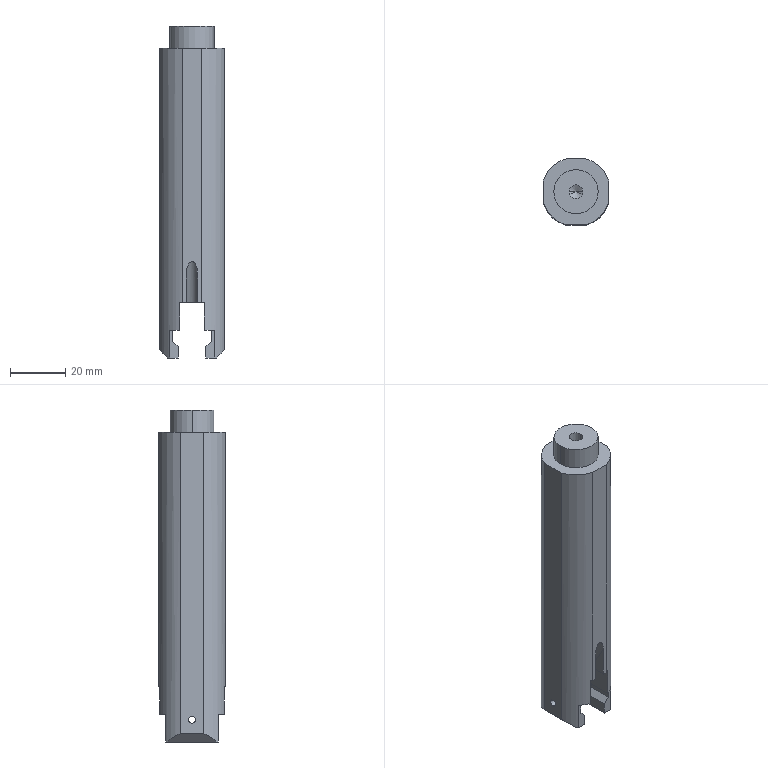Part | STEP file | magnetizing head 2 | 1 solid | 50 faces | box 23.5 x 24 x 120 mm | volume 49065 mm3 | plane 31 | cylinder 17 | cone 2 | commonest cylinder face diameters 2.5 x4 25 x4 10 x3 4 x2 5 x2 16 x2